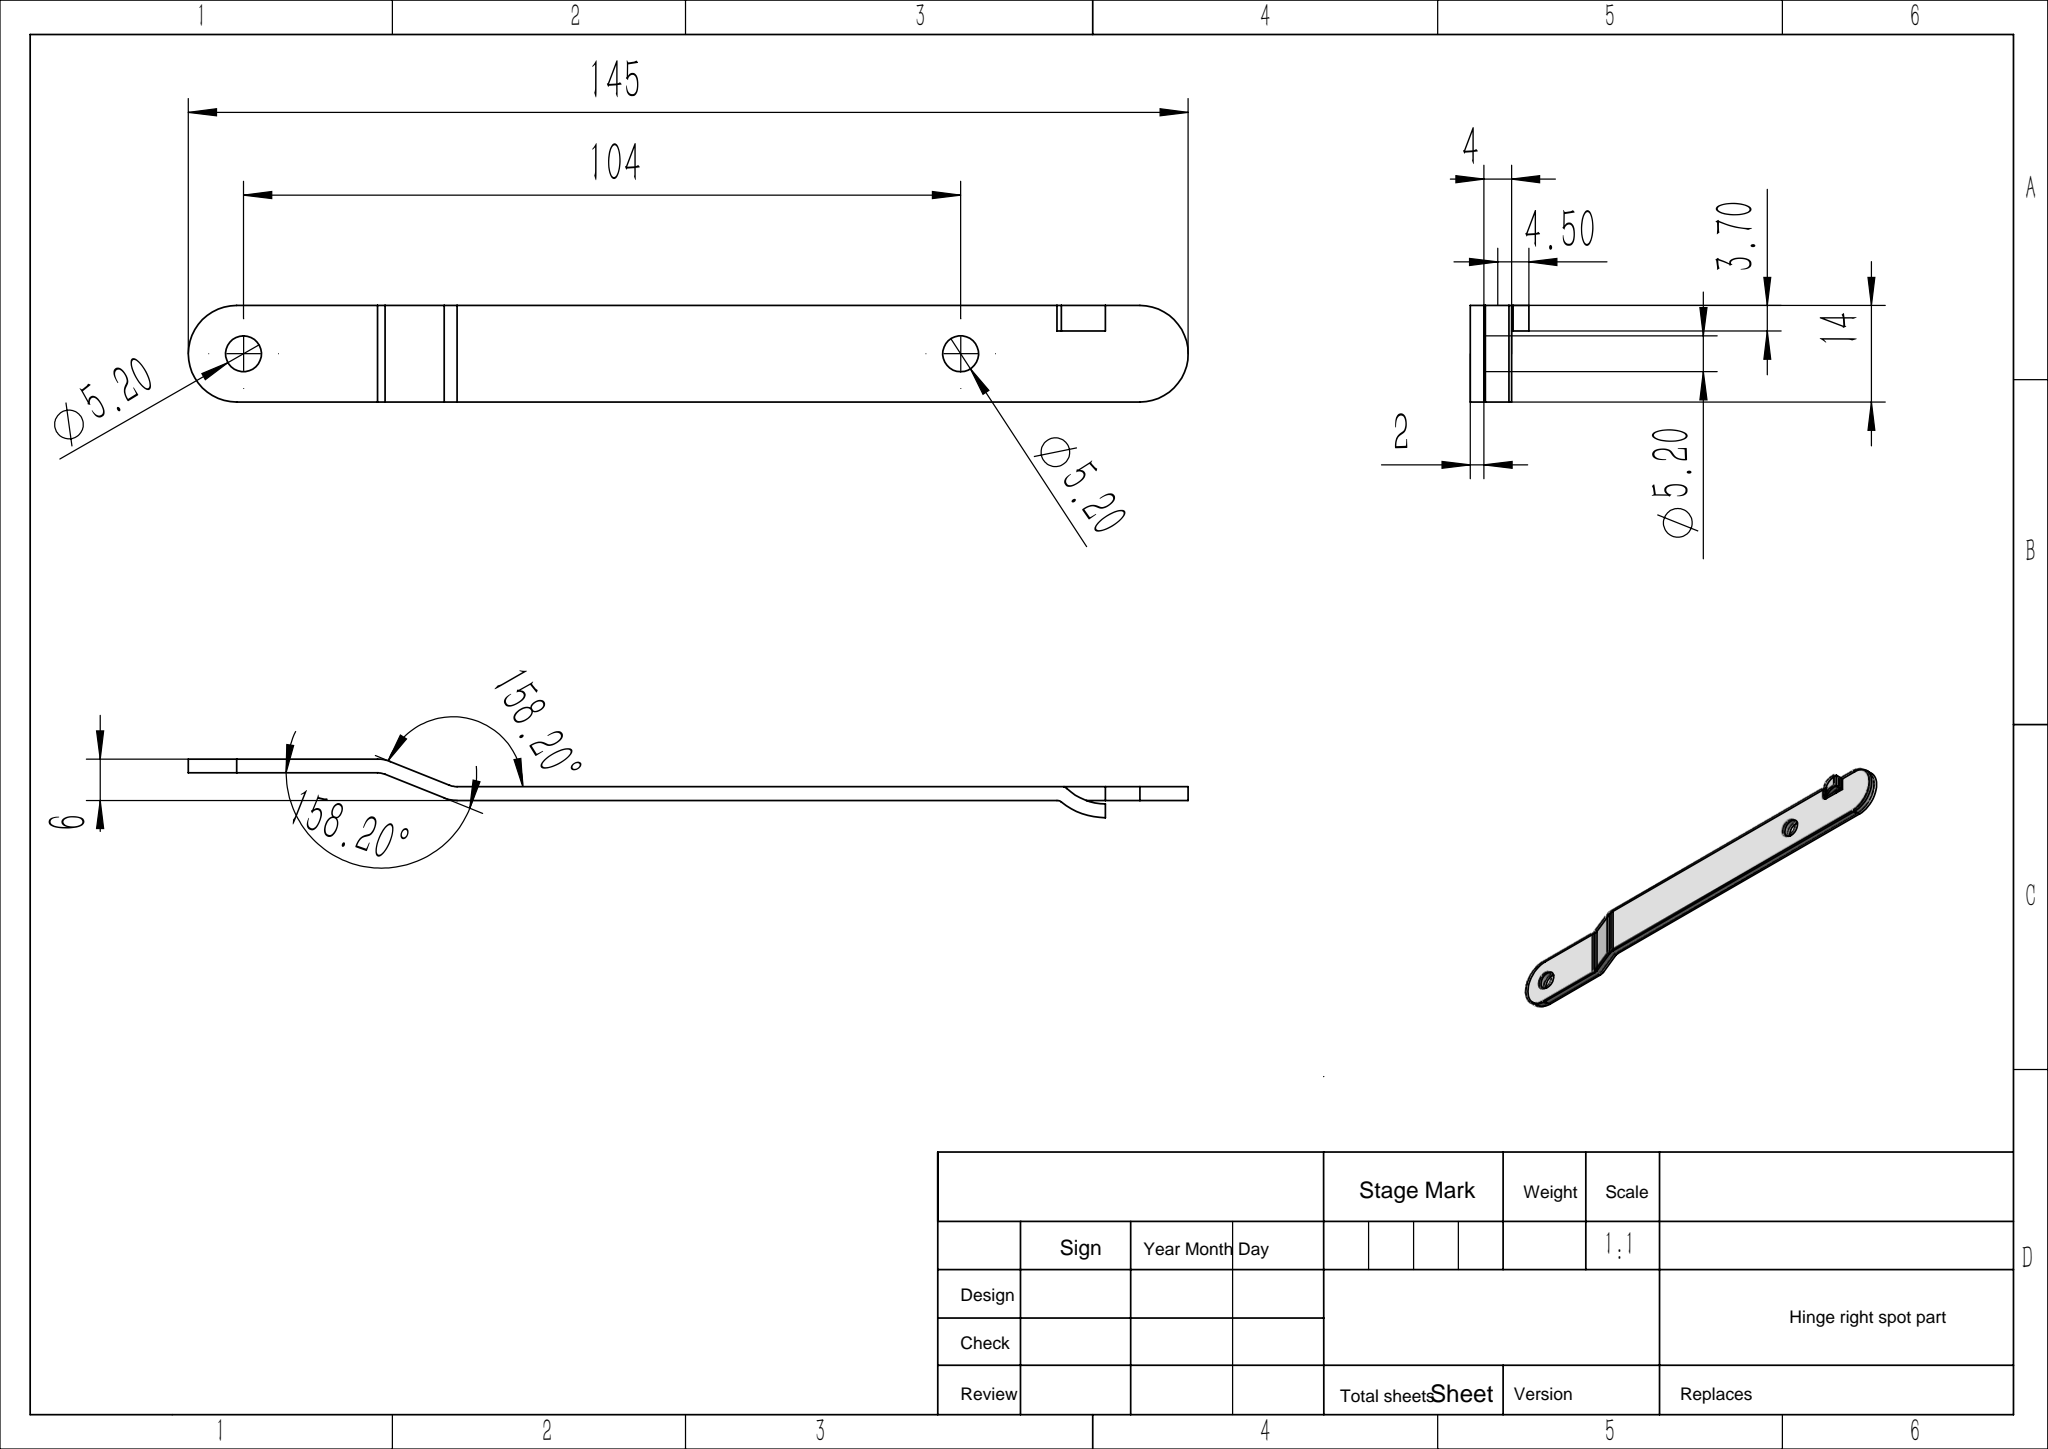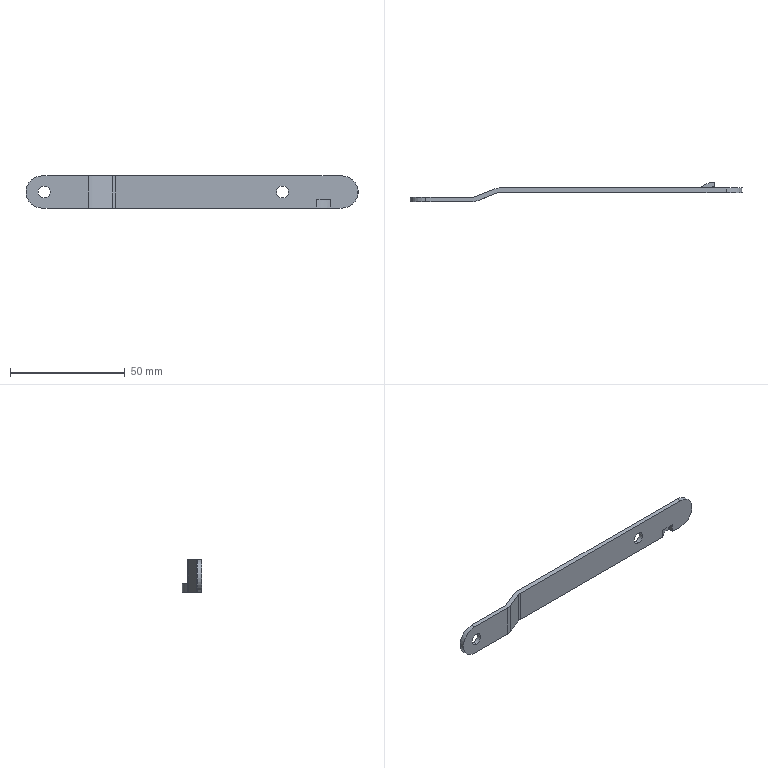Part | SolidWorks | features ICE 3, Extrusion 1 | 1 solid | 28 faces | box 145 x 8.5 x 14 mm | volume 3916 mm3 | cylinder 14 | plane 14 | commonest cylinder face diameters 5.2 x4 2 x2 6 x2 10 x2 14 x2 16.221 x1
STEP:
#1=CARTESIAN_POINT('',(112.,2.,-2.6));
#2=VERTEX_POINT('',#1);
#3=CARTESIAN_POINT('',(112.,2.,2.6));
#4=VERTEX_POINT('',#3);
#5=CARTESIAN_POINT('',(112.,2.,0.));
#6=DIRECTION('',(0.,1.,0.));
#7=DIRECTION('',(0.,0.,1.));
#8=AXIS2_PLACEMENT_3D('',#5,#6,#7);
#9=CIRCLE('',#8,2.6);
#10=EDGE_CURVE('',#2,#4,#9,.T.);
#11=ORIENTED_EDGE('',*,*,#10,.F.);
#12=CARTESIAN_POINT('',(112.,4.,-2.6));
#13=VERTEX_POINT('',#12);
#14=CARTESIAN_POINT('',(112.,-2.,-2.6));
#15=DIRECTION('',(0.,1.,0.));
#16=VECTOR('',#15,1000.);
#17=LINE('',#14,#16);
#18=EDGE_CURVE('',#2,#13,#17,.T.);
#19=ORIENTED_EDGE('',*,*,#18,.T.);
#20=CARTESIAN_POINT('',(112.,4.,2.6));
#21=VERTEX_POINT('',#20);
#22=CARTESIAN_POINT('',(112.,4.,0.));
#23=DIRECTION('',(0.,1.,0.));
#24=DIRECTION('',(0.,0.,1.));
#25=AXIS2_PLACEMENT_3D('',#22,#23,#24);
#26=CIRCLE('',#25,2.6);
#27=EDGE_CURVE('',#13,#21,#26,.T.);
#28=ORIENTED_EDGE('',*,*,#27,.T.);
#29=CARTESIAN_POINT('',(112.,-2.,2.6));
#30=DIRECTION('',(0.,1.,0.));
#31=VECTOR('',#30,1000.);
#32=LINE('',#29,#31);
#33=EDGE_CURVE('',#4,#21,#32,.T.);
#34=ORIENTED_EDGE('',*,*,#33,.F.);
#35=EDGE_LOOP('',(#11,#19,#28,#34));
#36=FACE_OUTER_BOUND('',#35,.T.);
#37=CARTESIAN_POINT('',(112.,-2.,0.));
#38=DIRECTION('',(0.,1.,0.));
#39=DIRECTION('',(0.,0.,1.));
#40=AXIS2_PLACEMENT_3D('',#37,#38,#39);
#41=CYLINDRICAL_SURFACE('',#40,2.6);
#42=ADVANCED_FACE('',(#36),#41,.F.);
#43=CARTESIAN_POINT('',(8.,-2.,-2.6));
#44=VERTEX_POINT('',#43);
#45=CARTESIAN_POINT('',(8.,-2.,2.6));
#46=VERTEX_POINT('',#45);
#47=CARTESIAN_POINT('',(8.,-2.,0.));
#48=DIRECTION('',(0.,1.,0.));
#49=DIRECTION('',(0.,0.,1.));
#50=AXIS2_PLACEMENT_3D('',#47,#48,#49);
#51=CIRCLE('',#50,2.6);
#52=EDGE_CURVE('',#44,#46,#51,.T.);
#53=ORIENTED_EDGE('',*,*,#52,.F.);
#54=CARTESIAN_POINT('',(8.,0.,-2.6));
#55=VERTEX_POINT('',#54);
#56=CARTESIAN_POINT('',(8.,-2.,-2.6));
#57=DIRECTION('',(0.,1.,0.));
#58=VECTOR('',#57,1000.);
#59=LINE('',#56,#58);
#60=EDGE_CURVE('',#44,#55,#59,.T.);
#61=ORIENTED_EDGE('',*,*,#60,.T.);
#62=CARTESIAN_POINT('',(8.,0.,2.6));
#63=VERTEX_POINT('',#62);
#64=CARTESIAN_POINT('',(8.,0.,0.));
#65=DIRECTION('',(0.,-1.,0.));
#66=DIRECTION('',(0.,0.,-1.));
#67=AXIS2_PLACEMENT_3D('',#64,#65,#66);
#68=CIRCLE('',#67,2.6);
#69=EDGE_CURVE('',#63,#55,#68,.T.);
#70=ORIENTED_EDGE('',*,*,#69,.F.);
#71=CARTESIAN_POINT('',(8.,-2.,2.6));
#72=DIRECTION('',(0.,1.,0.));
#73=VECTOR('',#72,1000.);
#74=LINE('',#71,#73);
#75=EDGE_CURVE('',#46,#63,#74,.T.);
#76=ORIENTED_EDGE('',*,*,#75,.F.);
#77=EDGE_LOOP('',(#53,#61,#70,#76));
#78=FACE_OUTER_BOUND('',#77,.T.);
#79=CARTESIAN_POINT('',(8.,-2.,0.));
#80=DIRECTION('',(0.,1.,0.));
#81=DIRECTION('',(0.,0.,1.));
#82=AXIS2_PLACEMENT_3D('',#79,#80,#81);
#83=CYLINDRICAL_SURFACE('',#82,2.6);
#84=ADVANCED_FACE('',(#78),#83,.F.);
#85=CARTESIAN_POINT('',(127.,2.037,-3.3));
#86=VERTEX_POINT('',#85);
#87=CARTESIAN_POINT('',(127.419,2.274,-3.3));
#88=VERTEX_POINT('',#87);
#89=CARTESIAN_POINT('',(126.731,3.,-3.3));
#90=DIRECTION('',(0.,0.,1.));
#91=DIRECTION('',(1.,0.,0.));
#92=AXIS2_PLACEMENT_3D('',#89,#90,#91);
#93=CIRCLE('',#92,1.);
#94=EDGE_CURVE('',#86,#88,#93,.T.);
#95=ORIENTED_EDGE('',*,*,#94,.T.);
#96=CARTESIAN_POINT('',(130.196,4.,-3.3));
#97=VERTEX_POINT('',#96);
#98=CARTESIAN_POINT('',(133.,-3.611,-3.3));
#99=DIRECTION('',(0.,0.,-1.));
#100=DIRECTION('',(-1.,0.,0.));
#101=AXIS2_PLACEMENT_3D('',#98,#99,#100);
#102=CIRCLE('',#101,8.111);
#103=EDGE_CURVE('',#88,#97,#102,.T.);
#104=ORIENTED_EDGE('',*,*,#103,.T.);
#105=CARTESIAN_POINT('',(133.,4.,-3.3));
#106=VERTEX_POINT('',#105);
#107=CARTESIAN_POINT('',(127.,4.,-3.3));
#108=DIRECTION('',(1.,0.,0.));
#109=VECTOR('',#108,1000.);
#110=LINE('',#107,#109);
#111=EDGE_CURVE('',#97,#106,#110,.T.);
#112=ORIENTED_EDGE('',*,*,#111,.T.);
#113=CARTESIAN_POINT('',(133.,2.,-3.3));
#114=VERTEX_POINT('',#113);
#115=CARTESIAN_POINT('',(133.,-2.,-3.3));
#116=DIRECTION('',(0.,1.,0.));
#117=VECTOR('',#116,1000.);
#118=LINE('',#115,#117);
#119=EDGE_CURVE('',#114,#106,#118,.T.);
#120=ORIENTED_EDGE('',*,*,#119,.F.);
#121=CARTESIAN_POINT('',(127.,2.,-3.3));
#122=VERTEX_POINT('',#121);
#123=CARTESIAN_POINT('',(38.963,2.,-3.3));
#124=DIRECTION('',(1.,0.,0.));
#125=VECTOR('',#124,1000.);
#126=LINE('',#123,#125);
#127=EDGE_CURVE('',#122,#114,#126,.T.);
#128=ORIENTED_EDGE('',*,*,#127,.F.);
#129=CARTESIAN_POINT('',(127.,-2.,-3.3));
#130=DIRECTION('',(0.,1.,0.));
#131=VECTOR('',#130,1000.);
#132=LINE('',#129,#131);
#133=EDGE_CURVE('',#122,#86,#132,.T.);
#134=ORIENTED_EDGE('',*,*,#133,.T.);
#135=EDGE_LOOP('',(#95,#104,#112,#120,#128,#134));
#136=FACE_OUTER_BOUND('',#135,.T.);
#137=CARTESIAN_POINT('',(127.,-2.,-3.3));
#138=DIRECTION('',(0.,0.,1.));
#139=DIRECTION('',(1.,0.,0.));
#140=AXIS2_PLACEMENT_3D('',#137,#138,#139);
#141=PLANE('',#140);
#142=ADVANCED_FACE('',(#136),#141,.F.);
#143=CARTESIAN_POINT('',(127.,2.037,-7.));
#144=VERTEX_POINT('',#143);
#145=CARTESIAN_POINT('',(127.,2.037,-3.3));
#146=DIRECTION('',(0.,0.,-1.));
#147=VECTOR('',#146,1000.);
#148=LINE('',#145,#147);
#149=EDGE_CURVE('',#86,#144,#148,.T.);
#150=ORIENTED_EDGE('',*,*,#149,.F.);
#151=ORIENTED_EDGE('',*,*,#133,.F.);
#152=CARTESIAN_POINT('',(127.,2.,-7.));
#153=VERTEX_POINT('',#152);
#154=CARTESIAN_POINT('',(127.,2.,7.));
#155=DIRECTION('',(0.,0.,1.));
#156=VECTOR('',#155,1000.);
#157=LINE('',#154,#156);
#158=EDGE_CURVE('',#153,#122,#157,.T.);
#159=ORIENTED_EDGE('',*,*,#158,.F.);
#160=CARTESIAN_POINT('',(127.,3.,-7.));
#161=DIRECTION('',(0.,1.,0.));
#162=VECTOR('',#161,1000.);
#163=LINE('',#160,#162);
#164=EDGE_CURVE('',#153,#144,#163,.T.);
#165=ORIENTED_EDGE('',*,*,#164,.T.);
#166=EDGE_LOOP('',(#150,#151,#159,#165));
#167=FACE_OUTER_BOUND('',#166,.T.);
#168=CARTESIAN_POINT('',(127.,-2.,-7.));
#169=DIRECTION('',(-1.,0.,0.));
#170=DIRECTION('',(0.,0.,1.));
#171=AXIS2_PLACEMENT_3D('',#168,#169,#170);
#172=PLANE('',#171);
#173=ADVANCED_FACE('',(#167),#172,.F.);
#174=CARTESIAN_POINT('',(125.978,4.,-7.));
#175=VERTEX_POINT('',#174);
#176=CARTESIAN_POINT('',(38.963,4.,-7.));
#177=VERTEX_POINT('',#176);
#178=CARTESIAN_POINT('',(38.963,4.,-7.));
#179=DIRECTION('',(-1.,0.,0.));
#180=VECTOR('',#179,1000.);
#181=LINE('',#178,#180);
#182=EDGE_CURVE('',#175,#177,#181,.T.);
#183=ORIENTED_EDGE('',*,*,#182,.F.);
#184=CARTESIAN_POINT('',(126.61,4.225,-7.));
#185=VERTEX_POINT('',#184);
#186=CARTESIAN_POINT('',(125.978,5.,-7.));
#187=DIRECTION('',(0.,0.,-1.));
#188=DIRECTION('',(1.,0.,0.));
#189=AXIS2_PLACEMENT_3D('',#186,#187,#188);
#190=CIRCLE('',#189,1.);
#191=EDGE_CURVE('',#185,#175,#190,.T.);
#192=ORIENTED_EDGE('',*,*,#191,.F.);
#193=CARTESIAN_POINT('',(133.,6.5,-7.));
#194=VERTEX_POINT('',#193);
#195=CARTESIAN_POINT('',(133.,-3.611,-7.));
#196=DIRECTION('',(0.,0.,1.));
#197=DIRECTION('',(-1.,0.,0.));
#198=AXIS2_PLACEMENT_3D('',#195,#196,#197);
#199=CIRCLE('',#198,10.111);
#200=EDGE_CURVE('',#194,#185,#199,.T.);
#201=ORIENTED_EDGE('',*,*,#200,.F.);
#202=CARTESIAN_POINT('',(133.,4.5,-7.));
#203=VERTEX_POINT('',#202);
#204=CARTESIAN_POINT('',(133.,4.5,-7.));
#205=DIRECTION('',(0.,1.,0.));
#206=VECTOR('',#205,1000.);
#207=LINE('',#204,#206);
#208=EDGE_CURVE('',#203,#194,#207,.T.);
#209=ORIENTED_EDGE('',*,*,#208,.F.);
#210=CARTESIAN_POINT('',(127.419,2.274,-7.));
#211=VERTEX_POINT('',#210);
#212=CARTESIAN_POINT('',(133.,-3.611,-7.));
#213=DIRECTION('',(0.,0.,-1.));
#214=DIRECTION('',(-1.,0.,0.));
#215=AXIS2_PLACEMENT_3D('',#212,#213,#214);
#216=CIRCLE('',#215,8.111);
#217=EDGE_CURVE('',#211,#203,#216,.T.);
#218=ORIENTED_EDGE('',*,*,#217,.F.);
#219=CARTESIAN_POINT('',(126.731,3.,-7.));
#220=DIRECTION('',(0.,0.,1.));
#221=DIRECTION('',(1.,0.,0.));
#222=AXIS2_PLACEMENT_3D('',#219,#220,#221);
#223=CIRCLE('',#222,1.);
#224=EDGE_CURVE('',#144,#211,#223,.T.);
#225=ORIENTED_EDGE('',*,*,#224,.F.);
#226=ORIENTED_EDGE('',*,*,#164,.F.);
#227=CARTESIAN_POINT('',(38.963,2.,-7.));
#228=VERTEX_POINT('',#227);
#229=CARTESIAN_POINT('',(38.963,2.,-7.));
#230=DIRECTION('',(1.,0.,0.));
#231=VECTOR('',#230,1000.);
#232=LINE('',#229,#231);
#233=EDGE_CURVE('',#228,#153,#232,.T.);
#234=ORIENTED_EDGE('',*,*,#233,.F.);
#235=CARTESIAN_POINT('',(37.849,1.785,-7.));
#236=VERTEX_POINT('',#235);
#237=CARTESIAN_POINT('',(38.963,-1.,-7.));
#238=DIRECTION('',(0.,0.,-1.));
#239=DIRECTION('',(1.,0.,0.));
#240=AXIS2_PLACEMENT_3D('',#237,#238,#239);
#241=CIRCLE('',#240,3.);
#242=EDGE_CURVE('',#236,#228,#241,.T.);
#243=ORIENTED_EDGE('',*,*,#242,.F.);
#244=CARTESIAN_POINT('',(29.279,-1.642,-7.));
#245=VERTEX_POINT('',#244);
#246=CARTESIAN_POINT('',(29.279,-1.642,-7.));
#247=DIRECTION('',(0.9285,0.3714,0.));
#248=VECTOR('',#247,1000.);
#249=LINE('',#246,#248);
#250=EDGE_CURVE('',#245,#236,#249,.T.);
#251=ORIENTED_EDGE('',*,*,#250,.F.);
#252=CARTESIAN_POINT('',(27.422,-2.,-7.));
#253=VERTEX_POINT('',#252);
#254=CARTESIAN_POINT('',(27.422,3.,-7.));
#255=DIRECTION('',(0.,0.,1.));
#256=DIRECTION('',(-1.,0.,0.));
#257=AXIS2_PLACEMENT_3D('',#254,#255,#256);
#258=CIRCLE('',#257,5.);
#259=EDGE_CURVE('',#253,#245,#258,.T.);
#260=ORIENTED_EDGE('',*,*,#259,.F.);
#261=CARTESIAN_POINT('',(7.,-2.,-7.));
#262=VERTEX_POINT('',#261);
#263=CARTESIAN_POINT('',(0.,-2.,-7.));
#264=DIRECTION('',(1.,0.,0.));
#265=VECTOR('',#264,1000.);
#266=LINE('',#263,#265);
#267=EDGE_CURVE('',#262,#253,#266,.T.);
#268=ORIENTED_EDGE('',*,*,#267,.F.);
#269=CARTESIAN_POINT('',(7.,0.,-7.));
#270=VERTEX_POINT('',#269);
#271=CARTESIAN_POINT('',(7.,-2.,-7.));
#272=DIRECTION('',(0.,1.,0.));
#273=VECTOR('',#272,1000.);
#274=LINE('',#271,#273);
#275=EDGE_CURVE('',#262,#270,#274,.T.);
#276=ORIENTED_EDGE('',*,*,#275,.T.);
#277=CARTESIAN_POINT('',(27.422,0.,-7.));
#278=VERTEX_POINT('',#277);
#279=CARTESIAN_POINT('',(0.,0.,-7.));
#280=DIRECTION('',(-1.,0.,0.));
#281=VECTOR('',#280,1000.);
#282=LINE('',#279,#281);
#283=EDGE_CURVE('',#278,#270,#282,.T.);
#284=ORIENTED_EDGE('',*,*,#283,.F.);
#285=CARTESIAN_POINT('',(28.536,0.2146,-7.));
#286=VERTEX_POINT('',#285);
#287=CARTESIAN_POINT('',(27.422,3.,-7.));
#288=DIRECTION('',(0.,0.,-1.));
#289=DIRECTION('',(-1.,0.,0.));
#290=AXIS2_PLACEMENT_3D('',#287,#288,#289);
#291=CIRCLE('',#290,3.);
#292=EDGE_CURVE('',#286,#278,#291,.T.);
#293=ORIENTED_EDGE('',*,*,#292,.F.);
#294=CARTESIAN_POINT('',(37.106,3.642,-7.));
#295=VERTEX_POINT('',#294);
#296=CARTESIAN_POINT('',(28.536,0.2146,-7.));
#297=DIRECTION('',(-0.9285,-0.3714,0.));
#298=VECTOR('',#297,1000.);
#299=LINE('',#296,#298);
#300=EDGE_CURVE('',#295,#286,#299,.T.);
#301=ORIENTED_EDGE('',*,*,#300,.F.);
#302=CARTESIAN_POINT('',(38.963,-1.,-7.));
#303=DIRECTION('',(0.,0.,1.));
#304=DIRECTION('',(1.,0.,0.));
#305=AXIS2_PLACEMENT_3D('',#302,#303,#304);
#306=CIRCLE('',#305,5.);
#307=EDGE_CURVE('',#177,#295,#306,.T.);
#308=ORIENTED_EDGE('',*,*,#307,.F.);
#309=EDGE_LOOP('',(#183,#192,#201,#209,#218,#225,#226,#234,#243,#251,#260,#268,#276,#284,#293,#301,#308));
#310=FACE_OUTER_BOUND('',#309,.T.);
#311=CARTESIAN_POINT('',(27.422,3.,-7.));
#312=DIRECTION('',(0.,0.,-1.));
#313=DIRECTION('',(-1.,0.,0.));
#314=AXIS2_PLACEMENT_3D('',#311,#312,#313);
#315=PLANE('',#314);
#316=ADVANCED_FACE('',(#310),#315,.T.);
#317=CARTESIAN_POINT('',(8.,-2.,0.));
#318=DIRECTION('',(0.,1.,0.));
#319=DIRECTION('',(0.,0.,1.));
#320=AXIS2_PLACEMENT_3D('',#317,#318,#319);
#321=CIRCLE('',#320,2.6);
#322=EDGE_CURVE('',#46,#44,#321,.T.);
#323=ORIENTED_EDGE('',*,*,#322,.T.);
#324=ORIENTED_EDGE('',*,*,#52,.T.);
#325=EDGE_LOOP('',(#323,#324));
#326=FACE_BOUND('',#325,.T.);
#327=CARTESIAN_POINT('',(7.,-2.,7.));
#328=VERTEX_POINT('',#327);
#329=CARTESIAN_POINT('',(27.422,-2.,7.));
#330=VERTEX_POINT('',#329);
#331=CARTESIAN_POINT('',(0.,-2.,7.));
#332=DIRECTION('',(1.,0.,0.));
#333=VECTOR('',#332,1000.);
#334=LINE('',#331,#333);
#335=EDGE_CURVE('',#328,#330,#334,.T.);
#336=ORIENTED_EDGE('',*,*,#335,.F.);
#337=CARTESIAN_POINT('',(7.,-2.,0.));
#338=DIRECTION('',(0.,-1.,0.));
#339=DIRECTION('',(0.,0.,1.));
#340=AXIS2_PLACEMENT_3D('',#337,#338,#339);
#341=CIRCLE('',#340,7.);
#342=EDGE_CURVE('',#328,#262,#341,.T.);
#343=ORIENTED_EDGE('',*,*,#342,.T.);
#344=ORIENTED_EDGE('',*,*,#267,.T.);
#345=CARTESIAN_POINT('',(27.422,-2.,7.));
#346=DIRECTION('',(0.,0.,-1.));
#347=VECTOR('',#346,1000.);
#348=LINE('',#345,#347);
#349=EDGE_CURVE('',#330,#253,#348,.T.);
#350=ORIENTED_EDGE('',*,*,#349,.F.);
#351=EDGE_LOOP('',(#336,#343,#344,#350));
#352=FACE_OUTER_BOUND('',#351,.T.);
#353=CARTESIAN_POINT('',(0.,-2.,7.));
#354=DIRECTION('',(0.,1.,0.));
#355=DIRECTION('',(0.,0.,1.));
#356=AXIS2_PLACEMENT_3D('',#353,#354,#355);
#357=PLANE('',#356);
#358=ADVANCED_FACE('',(#326,#352),#357,.F.);
#359=ORIENTED_EDGE('',*,*,#259,.T.);
#360=CARTESIAN_POINT('',(29.279,-1.642,7.));
#361=VERTEX_POINT('',#360);
#362=CARTESIAN_POINT('',(29.279,-1.642,7.));
#363=DIRECTION('',(0.,0.,-1.));
#364=VECTOR('',#363,1000.);
#365=LINE('',#362,#364);
#366=EDGE_CURVE('',#361,#245,#365,.T.);
#367=ORIENTED_EDGE('',*,*,#366,.F.);
#368=CARTESIAN_POINT('',(27.422,3.,7.));
#369=DIRECTION('',(0.,0.,1.));
#370=DIRECTION('',(-1.,0.,0.));
#371=AXIS2_PLACEMENT_3D('',#368,#369,#370);
#372=CIRCLE('',#371,5.);
#373=EDGE_CURVE('',#330,#361,#372,.T.);
#374=ORIENTED_EDGE('',*,*,#373,.F.);
#375=ORIENTED_EDGE('',*,*,#349,.T.);
#376=EDGE_LOOP('',(#359,#367,#374,#375));
#377=FACE_OUTER_BOUND('',#376,.T.);
#378=CARTESIAN_POINT('',(27.422,3.,7.));
#379=DIRECTION('',(0.,0.,-1.));
#380=DIRECTION('',(-1.,0.,0.));
#381=AXIS2_PLACEMENT_3D('',#378,#379,#380);
#382=CYLINDRICAL_SURFACE('',#381,5.);
#383=ADVANCED_FACE('',(#377),#382,.T.);
#384=ORIENTED_EDGE('',*,*,#250,.T.);
#385=CARTESIAN_POINT('',(37.849,1.785,7.));
#386=VERTEX_POINT('',#385);
#387=CARTESIAN_POINT('',(37.849,1.785,7.));
#388=DIRECTION('',(0.,0.,-1.));
#389=VECTOR('',#388,1000.);
#390=LINE('',#387,#389);
#391=EDGE_CURVE('',#386,#236,#390,.T.);
#392=ORIENTED_EDGE('',*,*,#391,.F.);
#393=CARTESIAN_POINT('',(29.279,-1.642,7.));
#394=DIRECTION('',(0.9285,0.3714,0.));
#395=VECTOR('',#394,1000.);
#396=LINE('',#393,#395);
#397=EDGE_CURVE('',#361,#386,#396,.T.);
#398=ORIENTED_EDGE('',*,*,#397,.F.);
#399=ORIENTED_EDGE('',*,*,#366,.T.);
#400=EDGE_LOOP('',(#384,#392,#398,#399));
#401=FACE_OUTER_BOUND('',#400,.T.);
#402=CARTESIAN_POINT('',(29.279,-1.642,7.));
#403=DIRECTION('',(-0.3714,0.9285,0.));
#404=DIRECTION('',(-0.9285,-0.3714,0.));
#405=AXIS2_PLACEMENT_3D('',#402,#403,#404);
#406=PLANE('',#405);
#407=ADVANCED_FACE('',(#401),#406,.F.);
#408=ORIENTED_EDGE('',*,*,#242,.T.);
#409=CARTESIAN_POINT('',(38.963,2.,7.));
#410=VERTEX_POINT('',#409);
#411=CARTESIAN_POINT('',(38.963,2.,7.));
#412=DIRECTION('',(0.,0.,-1.));
#413=VECTOR('',#412,1000.);
#414=LINE('',#411,#413);
#415=EDGE_CURVE('',#410,#228,#414,.T.);
#416=ORIENTED_EDGE('',*,*,#415,.F.);
#417=CARTESIAN_POINT('',(38.963,-1.,7.));
#418=DIRECTION('',(0.,0.,-1.));
#419=DIRECTION('',(1.,0.,0.));
#420=AXIS2_PLACEMENT_3D('',#417,#418,#419);
#421=CIRCLE('',#420,3.);
#422=EDGE_CURVE('',#386,#410,#421,.T.);
#423=ORIENTED_EDGE('',*,*,#422,.F.);
#424=ORIENTED_EDGE('',*,*,#391,.T.);
#425=EDGE_LOOP('',(#408,#416,#423,#424));
#426=FACE_OUTER_BOUND('',#425,.T.);
#427=CARTESIAN_POINT('',(38.963,-1.,7.));
#428=DIRECTION('',(0.,0.,-1.));
#429=DIRECTION('',(-1.,0.,0.));
#430=AXIS2_PLACEMENT_3D('',#427,#428,#429);
#431=CYLINDRICAL_SURFACE('',#430,3.);
#432=ADVANCED_FACE('',(#426),#431,.F.);
#433=ORIENTED_EDGE('',*,*,#233,.T.);
#434=ORIENTED_EDGE('',*,*,#158,.T.);
#435=ORIENTED_EDGE('',*,*,#127,.T.);
#436=CARTESIAN_POINT('',(133.,2.,-7.));
#437=VERTEX_POINT('',#436);
#438=CARTESIAN_POINT('',(133.,2.,7.));
#439=DIRECTION('',(0.,0.,-1.));
#440=VECTOR('',#439,1000.);
#441=LINE('',#438,#440);
#442=EDGE_CURVE('',#114,#437,#441,.T.);
#443=ORIENTED_EDGE('',*,*,#442,.T.);
#444=CARTESIAN_POINT('',(138.,2.,-7.));
#445=VERTEX_POINT('',#444);
#446=CARTESIAN_POINT('',(38.963,2.,-7.));
#447=DIRECTION('',(1.,0.,0.));
#448=VECTOR('',#447,1000.);
#449=LINE('',#446,#448);
#450=EDGE_CURVE('',#437,#445,#449,.T.);
#451=ORIENTED_EDGE('',*,*,#450,.T.);
#452=CARTESIAN_POINT('',(138.,2.,7.));
#453=VERTEX_POINT('',#452);
#454=CARTESIAN_POINT('',(138.,2.,0.));
#455=DIRECTION('',(0.,-1.,0.));
#456=DIRECTION('',(0.,0.,1.));
#457=AXIS2_PLACEMENT_3D('',#454,#455,#456);
#458=CIRCLE('',#457,7.);
#459=EDGE_CURVE('',#445,#453,#458,.T.);
#460=ORIENTED_EDGE('',*,*,#459,.T.);
#461=CARTESIAN_POINT('',(38.963,2.,7.));
#462=DIRECTION('',(1.,0.,0.));
#463=VECTOR('',#462,1000.);
#464=LINE('',#461,#463);
#465=EDGE_CURVE('',#410,#453,#464,.T.);
#466=ORIENTED_EDGE('',*,*,#465,.F.);
#467=ORIENTED_EDGE('',*,*,#415,.T.);
#468=EDGE_LOOP('',(#433,#434,#435,#443,#451,#460,#466,#467));
#469=FACE_OUTER_BOUND('',#468,.T.);
#470=CARTESIAN_POINT('',(112.,2.,0.));
#471=DIRECTION('',(0.,1.,0.));
#472=DIRECTION('',(0.,0.,1.));
#473=AXIS2_PLACEMENT_3D('',#470,#471,#472);
#474=CIRCLE('',#473,2.6);
#475=EDGE_CURVE('',#4,#2,#474,.T.);
#476=ORIENTED_EDGE('',*,*,#475,.T.);
#477=ORIENTED_EDGE('',*,*,#10,.T.);
#478=EDGE_LOOP('',(#476,#477));
#479=FACE_BOUND('',#478,.T.);
#480=CARTESIAN_POINT('',(38.963,2.,7.));
#481=DIRECTION('',(0.,1.,0.));
#482=DIRECTION('',(0.,0.,1.));
#483=AXIS2_PLACEMENT_3D('',#480,#481,#482);
#484=PLANE('',#483);
#485=ADVANCED_FACE('',(#469,#479),#484,.F.);
#486=ORIENTED_EDGE('',*,*,#182,.T.);
#487=CARTESIAN_POINT('',(38.963,4.,7.));
#488=VERTEX_POINT('',#487);
#489=CARTESIAN_POINT('',(38.963,4.,7.));
#490=DIRECTION('',(0.,0.,-1.));
#491=VECTOR('',#490,1000.);
#492=LINE('',#489,#491);
#493=EDGE_CURVE('',#488,#177,#492,.T.);
#494=ORIENTED_EDGE('',*,*,#493,.F.);
#495=CARTESIAN_POINT('',(138.,4.,7.));
#496=VERTEX_POINT('',#495);
#497=CARTESIAN_POINT('',(38.963,4.,7.));
#498=DIRECTION('',(-1.,0.,0.));
#499=VECTOR('',#498,1000.);
#500=LINE('',#497,#499);
#501=EDGE_CURVE('',#496,#488,#500,.T.);
#502=ORIENTED_EDGE('',*,*,#501,.F.);
#503=CARTESIAN_POINT('',(138.,4.,-7.));
#504=VERTEX_POINT('',#503);
#505=CARTESIAN_POINT('',(138.,4.,0.));
#506=DIRECTION('',(0.,-1.,0.));
#507=DIRECTION('',(0.,0.,1.));
#508=AXIS2_PLACEMENT_3D('',#505,#506,#507);
#509=CIRCLE('',#508,7.);
#510=EDGE_CURVE('',#504,#496,#509,.T.);
#511=ORIENTED_EDGE('',*,*,#510,.F.);
#512=CARTESIAN_POINT('',(133.,4.,-7.));
#513=VERTEX_POINT('',#512);
#514=CARTESIAN_POINT('',(38.963,4.,-7.));
#515=DIRECTION('',(-1.,0.,0.));
#516=VECTOR('',#515,1000.);
#517=LINE('',#514,#516);
#518=EDGE_CURVE('',#504,#513,#517,.T.);
#519=ORIENTED_EDGE('',*,*,#518,.T.);
#520=CARTESIAN_POINT('',(133.,4.,-7.));
#521=DIRECTION('',(0.,0.,-1.));
#522=VECTOR('',#521,1000.);
#523=LINE('',#520,#522);
#524=EDGE_CURVE('',#106,#513,#523,.T.);
#525=ORIENTED_EDGE('',*,*,#524,.F.);
#526=ORIENTED_EDGE('',*,*,#111,.F.);
#527=CARTESIAN_POINT('',(125.978,4.,-3.3));
#528=VERTEX_POINT('',#527);
#529=CARTESIAN_POINT('',(127.,4.,-3.3));
#530=DIRECTION('',(1.,0.,0.));
#531=VECTOR('',#530,1000.);
#532=LINE('',#529,#531);
#533=EDGE_CURVE('',#528,#97,#532,.T.);
#534=ORIENTED_EDGE('',*,*,#533,.F.);
#535=CARTESIAN_POINT('',(125.978,4.,-3.3));
#536=DIRECTION('',(0.,0.,-1.));
#537=VECTOR('',#536,1000.);
#538=LINE('',#535,#537);
#539=EDGE_CURVE('',#528,#175,#538,.T.);
#540=ORIENTED_EDGE('',*,*,#539,.T.);
#541=EDGE_LOOP('',(#486,#494,#502,#511,#519,#525,#526,#534,#540));
#542=FACE_OUTER_BOUND('',#541,.T.);
#543=CARTESIAN_POINT('',(112.,4.,0.));
#544=DIRECTION('',(0.,1.,0.));
#545=DIRECTION('',(0.,0.,1.));
#546=AXIS2_PLACEMENT_3D('',#543,#544,#545);
#547=CIRCLE('',#546,2.6);
#548=EDGE_CURVE('',#21,#13,#547,.T.);
#549=ORIENTED_EDGE('',*,*,#548,.F.);
#550=ORIENTED_EDGE('',*,*,#27,.F.);
#551=EDGE_LOOP('',(#549,#550));
#552=FACE_BOUND('',#551,.T.);
#553=CARTESIAN_POINT('',(38.963,4.,7.));
#554=DIRECTION('',(0.,-1.,0.));
#555=DIRECTION('',(0.,0.,-1.));
#556=AXIS2_PLACEMENT_3D('',#553,#554,#555);
#557=PLANE('',#556);
#558=ADVANCED_FACE('',(#542,#552),#557,.F.);
#559=ORIENTED_EDGE('',*,*,#307,.T.);
#560=CARTESIAN_POINT('',(37.106,3.642,7.));
#561=VERTEX_POINT('',#560);
#562=CARTESIAN_POINT('',(37.106,3.642,7.));
#563=DIRECTION('',(0.,0.,-1.));
#564=VECTOR('',#563,1000.);
#565=LINE('',#562,#564);
#566=EDGE_CURVE('',#561,#295,#565,.T.);
#567=ORIENTED_EDGE('',*,*,#566,.F.);
#568=CARTESIAN_POINT('',(38.963,-1.,7.));
#569=DIRECTION('',(0.,0.,1.));
#570=DIRECTION('',(1.,0.,0.));
#571=AXIS2_PLACEMENT_3D('',#568,#569,#570);
#572=CIRCLE('',#571,5.);
#573=EDGE_CURVE('',#488,#561,#572,.T.);
#574=ORIENTED_EDGE('',*,*,#573,.F.);
#575=ORIENTED_EDGE('',*,*,#493,.T.);
#576=EDGE_LOOP('',(#559,#567,#574,#575));
#577=FACE_OUTER_BOUND('',#576,.T.);
#578=CARTESIAN_POINT('',(38.963,-1.,7.));
#579=DIRECTION('',(0.,0.,-1.));
#580=DIRECTION('',(-1.,0.,0.));
#581=AXIS2_PLACEMENT_3D('',#578,#579,#580);
#582=CYLINDRICAL_SURFACE('',#581,5.);
#583=ADVANCED_FACE('',(#577),#582,.T.);
#584=ORIENTED_EDGE('',*,*,#300,.T.);
#585=CARTESIAN_POINT('',(28.536,0.2146,7.));
#586=VERTEX_POINT('',#585);
#587=CARTESIAN_POINT('',(28.536,0.2146,7.));
#588=DIRECTION('',(0.,0.,-1.));
#589=VECTOR('',#588,1000.);
#590=LINE('',#587,#589);
#591=EDGE_CURVE('',#586,#286,#590,.T.);
#592=ORIENTED_EDGE('',*,*,#591,.F.);
#593=CARTESIAN_POINT('',(28.536,0.2146,7.));
#594=DIRECTION('',(-0.9285,-0.3714,0.));
#595=VECTOR('',#594,1000.);
#596=LINE('',#593,#595);
#597=EDGE_CURVE('',#561,#586,#596,.T.);
#598=ORIENTED_EDGE('',*,*,#597,.F.);
#599=ORIENTED_EDGE('',*,*,#566,.T.);
#600=EDGE_LOOP('',(#584,#592,#598,#599));
#601=FACE_OUTER_BOUND('',#600,.T.);
#602=CARTESIAN_POINT('',(28.536,0.2146,7.));
#603=DIRECTION('',(0.3714,-0.9285,0.));
#604=DIRECTION('',(0.9285,0.3714,0.));
#605=AXIS2_PLACEMENT_3D('',#602,#603,#604);
#606=PLANE('',#605);
#607=ADVANCED_FACE('',(#601),#606,.F.);
#608=ORIENTED_EDGE('',*,*,#292,.T.);
#609=CARTESIAN_POINT('',(27.422,0.,7.));
#610=VERTEX_POINT('',#609);
#611=CARTESIAN_POINT('',(27.422,0.,7.));
#612=DIRECTION('',(0.,0.,-1.));
#613=VECTOR('',#612,1000.);
#614=LINE('',#611,#613);
#615=EDGE_CURVE('',#610,#278,#614,.T.);
#616=ORIENTED_EDGE('',*,*,#615,.F.);
#617=CARTESIAN_POINT('',(27.422,3.,7.));
#618=DIRECTION('',(0.,0.,-1.));
#619=DIRECTION('',(-1.,0.,0.));
#620=AXIS2_PLACEMENT_3D('',#617,#618,#619);
#621=CIRCLE('',#620,3.);
#622=EDGE_CURVE('',#586,#610,#621,.T.);
#623=ORIENTED_EDGE('',*,*,#622,.F.);
#624=ORIENTED_EDGE('',*,*,#591,.T.);
#625=EDGE_LOOP('',(#608,#616,#623,#624));
#626=FACE_OUTER_BOUND('',#625,.T.);
#627=CARTESIAN_POINT('',(27.422,3.,7.));
#628=DIRECTION('',(0.,0.,-1.));
#629=DIRECTION('',(-1.,0.,0.));
#630=AXIS2_PLACEMENT_3D('',#627,#628,#629);
#631=CYLINDRICAL_SURFACE('',#630,3.);
#632=ADVANCED_FACE('',(#626),#631,.F.);
#633=ORIENTED_EDGE('',*,*,#69,.T.);
#634=CARTESIAN_POINT('',(8.,0.,0.));
#635=DIRECTION('',(0.,-1.,0.));
#636=DIRECTION('',(0.,0.,-1.));
#637=AXIS2_PLACEMENT_3D('',#634,#635,#636);
#638=CIRCLE('',#637,2.6);
#639=EDGE_CURVE('',#55,#63,#638,.T.);
#640=ORIENTED_EDGE('',*,*,#639,.T.);
#641=EDGE_LOOP('',(#633,#640));
#642=FACE_BOUND('',#641,.T.);
#643=ORIENTED_EDGE('',*,*,#283,.T.);
#644=CARTESIAN_POINT('',(7.,0.,7.));
#645=VERTEX_POINT('',#644);
#646=CARTESIAN_POINT('',(7.,0.,0.));
#647=DIRECTION('',(0.,1.,0.));
#648=DIRECTION('',(0.,0.,-1.));
#649=AXIS2_PLACEMENT_3D('',#646,#647,#648);
#650=CIRCLE('',#649,7.);
#651=EDGE_CURVE('',#270,#645,#650,.T.);
#652=ORIENTED_EDGE('',*,*,#651,.T.);
#653=CARTESIAN_POINT('',(0.,0.,7.));
#654=DIRECTION('',(-1.,0.,0.));
#655=VECTOR('',#654,1000.);
#656=LINE('',#653,#655);
#657=EDGE_CURVE('',#610,#645,#656,.T.);
#658=ORIENTED_EDGE('',*,*,#657,.F.);
#659=ORIENTED_EDGE('',*,*,#615,.T.);
#660=EDGE_LOOP('',(#643,#652,#658,#659));
#661=FACE_OUTER_BOUND('',#660,.T.);
#662=CARTESIAN_POINT('',(0.,0.,7.));
#663=DIRECTION('',(0.,-1.,0.));
#664=DIRECTION('',(0.,0.,-1.));
#665=AXIS2_PLACEMENT_3D('',#662,#663,#664);
#666=PLANE('',#665);
#667=ADVANCED_FACE('',(#642,#661),#666,.F.);
#668=ORIENTED_EDGE('',*,*,#465,.T.);
#669=CARTESIAN_POINT('',(138.,-2.,7.));
#670=DIRECTION('',(0.,1.,0.));
#671=VECTOR('',#670,1000.);
#672=LINE('',#669,#671);
#673=EDGE_CURVE('',#453,#496,#672,.T.);
#674=ORIENTED_EDGE('',*,*,#673,.T.);
#675=ORIENTED_EDGE('',*,*,#501,.T.);
#676=ORIENTED_EDGE('',*,*,#573,.T.);
#677=ORIENTED_EDGE('',*,*,#597,.T.);
#678=ORIENTED_EDGE('',*,*,#622,.T.);
#679=ORIENTED_EDGE('',*,*,#657,.T.);
#680=CARTESIAN_POINT('',(7.,-2.,7.));
#681=DIRECTION('',(0.,1.,0.));
#682=VECTOR('',#681,1000.);
#683=LINE('',#680,#682);
#684=EDGE_CURVE('',#328,#645,#683,.T.);
#685=ORIENTED_EDGE('',*,*,#684,.F.);
#686=ORIENTED_EDGE('',*,*,#335,.T.);
#687=ORIENTED_EDGE('',*,*,#373,.T.);
#688=ORIENTED_EDGE('',*,*,#397,.T.);
#689=ORIENTED_EDGE('',*,*,#422,.T.);
#690=EDGE_LOOP('',(#668,#674,#675,#676,#677,#678,#679,#685,#686,#687,#688,#689));
#691=FACE_OUTER_BOUND('',#690,.T.);
#692=CARTESIAN_POINT('',(27.422,3.,7.));
#693=DIRECTION('',(0.,0.,-1.));
#694=DIRECTION('',(-1.,0.,0.));
#695=AXIS2_PLACEMENT_3D('',#692,#693,#694);
#696=PLANE('',#695);
#697=ADVANCED_FACE('',(#691),#696,.F.);
#698=CARTESIAN_POINT('',(133.,3.,-7.));
#699=DIRECTION('',(0.,-1.,0.));
#700=VECTOR('',#699,1000.);
#701=LINE('',#698,#700);
#702=EDGE_CURVE('',#513,#437,#701,.T.);
#703=ORIENTED_EDGE('',*,*,#702,.F.);
#704=ORIENTED_EDGE('',*,*,#518,.F.);
#705=CARTESIAN_POINT('',(138.,3.,-7.));
#706=DIRECTION('',(0.,1.,0.));
#707=VECTOR('',#706,1000.);
#708=LINE('',#705,#707);
#709=EDGE_CURVE('',#445,#504,#708,.T.);
#710=ORIENTED_EDGE('',*,*,#709,.F.);
#711=ORIENTED_EDGE('',*,*,#450,.F.);
#712=EDGE_LOOP('',(#703,#704,#710,#711));
#713=FACE_OUTER_BOUND('',#712,.T.);
#714=CARTESIAN_POINT('',(27.422,3.,-7.));
#715=DIRECTION('',(0.,0.,-1.));
#716=DIRECTION('',(-1.,0.,0.));
#717=AXIS2_PLACEMENT_3D('',#714,#715,#716);
#718=PLANE('',#717);
#719=ADVANCED_FACE('',(#713),#718,.T.);
#720=ORIENTED_EDGE('',*,*,#651,.F.);
#721=ORIENTED_EDGE('',*,*,#275,.F.);
#722=ORIENTED_EDGE('',*,*,#342,.F.);
#723=ORIENTED_EDGE('',*,*,#684,.T.);
#724=EDGE_LOOP('',(#720,#721,#722,#723));
#725=FACE_OUTER_BOUND('',#724,.T.);
#726=CARTESIAN_POINT('',(7.,-2.,0.));
#727=DIRECTION('',(0.,1.,0.));
#728=DIRECTION('',(0.,0.,1.));
#729=AXIS2_PLACEMENT_3D('',#726,#727,#728);
#730=CYLINDRICAL_SURFACE('',#729,7.);
#731=ADVANCED_FACE('',(#725),#730,.T.);
#732=ORIENTED_EDGE('',*,*,#709,.T.);
#733=ORIENTED_EDGE('',*,*,#510,.T.);
#734=ORIENTED_EDGE('',*,*,#673,.F.);
#735=ORIENTED_EDGE('',*,*,#459,.F.);
#736=EDGE_LOOP('',(#732,#733,#734,#735));
#737=FACE_OUTER_BOUND('',#736,.T.);
#738=CARTESIAN_POINT('',(138.,-2.,0.));
#739=DIRECTION('',(0.,1.,0.));
#740=DIRECTION('',(0.,0.,1.));
#741=AXIS2_PLACEMENT_3D('',#738,#739,#740);
#742=CYLINDRICAL_SURFACE('',#741,7.);
#743=ADVANCED_FACE('',(#737),#742,.T.);
#744=ORIENTED_EDGE('',*,*,#60,.F.);
#745=ORIENTED_EDGE('',*,*,#322,.F.);
#746=ORIENTED_EDGE('',*,*,#75,.T.);
#747=ORIENTED_EDGE('',*,*,#639,.F.);
#748=EDGE_LOOP('',(#744,#745,#746,#747));
#749=FACE_OUTER_BOUND('',#748,.T.);
#750=CARTESIAN_POINT('',(8.,-2.,0.));
#751=DIRECTION('',(0.,1.,0.));
#752=DIRECTION('',(0.,0.,1.));
#753=AXIS2_PLACEMENT_3D('',#750,#751,#752);
#754=CYLINDRICAL_SURFACE('',#753,2.6);
#755=ADVANCED_FACE('',(#749),#754,.F.);
#756=ORIENTED_EDGE('',*,*,#18,.F.);
#757=ORIENTED_EDGE('',*,*,#475,.F.);
#758=ORIENTED_EDGE('',*,*,#33,.T.);
#759=ORIENTED_EDGE('',*,*,#548,.T.);
#760=EDGE_LOOP('',(#756,#757,#758,#759));
#761=FACE_OUTER_BOUND('',#760,.T.);
#762=CARTESIAN_POINT('',(112.,-2.,0.));
#763=DIRECTION('',(0.,1.,0.));
#764=DIRECTION('',(0.,0.,1.));
#765=AXIS2_PLACEMENT_3D('',#762,#763,#764);
#766=CYLINDRICAL_SURFACE('',#765,2.6);
#767=ADVANCED_FACE('',(#761),#766,.F.);
#768=ORIENTED_EDGE('',*,*,#119,.T.);
#769=ORIENTED_EDGE('',*,*,#524,.T.);
#770=ORIENTED_EDGE('',*,*,#702,.T.);
#771=ORIENTED_EDGE('',*,*,#442,.F.);
#772=EDGE_LOOP('',(#768,#769,#770,#771));
#773=FACE_OUTER_BOUND('',#772,.T.);
#774=CARTESIAN_POINT('',(133.,-2.,-7.));
#775=DIRECTION('',(1.,0.,0.));
#776=DIRECTION('',(0.,0.,-1.));
#777=AXIS2_PLACEMENT_3D('',#774,#775,#776);
#778=PLANE('',#777);
#779=ADVANCED_FACE('',(#773),#778,.F.);
#780=ORIENTED_EDGE('',*,*,#94,.F.);
#781=ORIENTED_EDGE('',*,*,#149,.T.);
#782=ORIENTED_EDGE('',*,*,#224,.T.);
#783=CARTESIAN_POINT('',(127.419,2.274,-3.3));
#784=DIRECTION('',(0.,0.,-1.));
#785=VECTOR('',#784,1000.);
#786=LINE('',#783,#785);
#787=EDGE_CURVE('',#88,#211,#786,.T.);
#788=ORIENTED_EDGE('',*,*,#787,.F.);
#789=EDGE_LOOP('',(#780,#781,#782,#788));
#790=FACE_OUTER_BOUND('',#789,.T.);
#791=CARTESIAN_POINT('',(126.731,3.,-3.3));
#792=DIRECTION('',(0.,0.,-1.));
#793=DIRECTION('',(-1.,0.,0.));
#794=AXIS2_PLACEMENT_3D('',#791,#792,#793);
#795=CYLINDRICAL_SURFACE('',#794,1.);
#796=ADVANCED_FACE('',(#790),#795,.T.);
#797=CARTESIAN_POINT('',(126.61,4.225,-3.3));
#798=VERTEX_POINT('',#797);
#799=CARTESIAN_POINT('',(125.978,5.,-3.3));
#800=DIRECTION('',(0.,0.,-1.));
#801=DIRECTION('',(1.,0.,0.));
#802=AXIS2_PLACEMENT_3D('',#799,#800,#801);
#803=CIRCLE('',#802,1.);
#804=EDGE_CURVE('',#798,#528,#803,.T.);
#805=ORIENTED_EDGE('',*,*,#804,.T.);
#806=ORIENTED_EDGE('',*,*,#533,.T.);
#807=CARTESIAN_POINT('',(133.,4.5,-3.3));
#808=VERTEX_POINT('',#807);
#809=CARTESIAN_POINT('',(133.,-3.611,-3.3));
#810=DIRECTION('',(0.,0.,-1.));
#811=DIRECTION('',(-1.,0.,0.));
#812=AXIS2_PLACEMENT_3D('',#809,#810,#811);
#813=CIRCLE('',#812,8.111);
#814=EDGE_CURVE('',#97,#808,#813,.T.);
#815=ORIENTED_EDGE('',*,*,#814,.T.);
#816=CARTESIAN_POINT('',(133.,6.5,-3.3));
#817=VERTEX_POINT('',#816);
#818=CARTESIAN_POINT('',(133.,4.5,-3.3));
#819=DIRECTION('',(0.,1.,0.));
#820=VECTOR('',#819,1000.);
#821=LINE('',#818,#820);
#822=EDGE_CURVE('',#808,#817,#821,.T.);
#823=ORIENTED_EDGE('',*,*,#822,.T.);
#824=CARTESIAN_POINT('',(133.,-3.611,-3.3));
#825=DIRECTION('',(0.,0.,1.));
#826=DIRECTION('',(-1.,0.,0.));
#827=AXIS2_PLACEMENT_3D('',#824,#825,#826);
#828=CIRCLE('',#827,10.111);
#829=EDGE_CURVE('',#817,#798,#828,.T.);
#830=ORIENTED_EDGE('',*,*,#829,.T.);
#831=EDGE_LOOP('',(#805,#806,#815,#823,#830));
#832=FACE_OUTER_BOUND('',#831,.T.);
#833=CARTESIAN_POINT('',(133.,-3.611,-3.3));
#834=DIRECTION('',(0.,0.,-1.));
#835=DIRECTION('',(-1.,0.,0.));
#836=AXIS2_PLACEMENT_3D('',#833,#834,#835);
#837=PLANE('',#836);
#838=ADVANCED_FACE('',(#832),#837,.F.);
#839=ORIENTED_EDGE('',*,*,#200,.T.);
#840=CARTESIAN_POINT('',(126.61,4.225,-3.3));
#841=DIRECTION('',(0.,0.,-1.));
#842=VECTOR('',#841,1000.);
#843=LINE('',#840,#842);
#844=EDGE_CURVE('',#798,#185,#843,.T.);
#845=ORIENTED_EDGE('',*,*,#844,.F.);
#846=ORIENTED_EDGE('',*,*,#829,.F.);
#847=CARTESIAN_POINT('',(133.,6.5,-3.3));
#848=DIRECTION('',(0.,0.,-1.));
#849=VECTOR('',#848,1000.);
#850=LINE('',#847,#849);
#851=EDGE_CURVE('',#817,#194,#850,.T.);
#852=ORIENTED_EDGE('',*,*,#851,.T.);
#853=EDGE_LOOP('',(#839,#845,#846,#852));
#854=FACE_OUTER_BOUND('',#853,.T.);
#855=CARTESIAN_POINT('',(133.,-3.611,-3.3));
#856=DIRECTION('',(0.,0.,-1.));
#857=DIRECTION('',(-1.,0.,0.));
#858=AXIS2_PLACEMENT_3D('',#855,#856,#857);
#859=CYLINDRICAL_SURFACE('',#858,10.111);
#860=ADVANCED_FACE('',(#854),#859,.T.);
#861=ORIENTED_EDGE('',*,*,#191,.T.);
#862=ORIENTED_EDGE('',*,*,#539,.F.);
#863=ORIENTED_EDGE('',*,*,#804,.F.);
#864=ORIENTED_EDGE('',*,*,#844,.T.);
#865=EDGE_LOOP('',(#861,#862,#863,#864));
#866=FACE_OUTER_BOUND('',#865,.T.);
#867=CARTESIAN_POINT('',(125.978,5.,-3.3));
#868=DIRECTION('',(0.,0.,-1.));
#869=DIRECTION('',(-1.,0.,0.));
#870=AXIS2_PLACEMENT_3D('',#867,#868,#869);
#871=CYLINDRICAL_SURFACE('',#870,1.);
#872=ADVANCED_FACE('',(#866),#871,.F.);
#873=ORIENTED_EDGE('',*,*,#217,.T.);
#874=CARTESIAN_POINT('',(133.,4.5,-3.3));
#875=DIRECTION('',(0.,0.,-1.));
#876=VECTOR('',#875,1000.);
#877=LINE('',#874,#876);
#878=EDGE_CURVE('',#808,#203,#877,.T.);
#879=ORIENTED_EDGE('',*,*,#878,.F.);
#880=ORIENTED_EDGE('',*,*,#814,.F.);
#881=ORIENTED_EDGE('',*,*,#103,.F.);
#882=ORIENTED_EDGE('',*,*,#787,.T.);
#883=EDGE_LOOP('',(#873,#879,#880,#881,#882));
#884=FACE_OUTER_BOUND('',#883,.T.);
#885=CARTESIAN_POINT('',(133.,-3.611,-3.3));
#886=DIRECTION('',(0.,0.,-1.));
#887=DIRECTION('',(-1.,0.,0.));
#888=AXIS2_PLACEMENT_3D('',#885,#886,#887);
#889=CYLINDRICAL_SURFACE('',#888,8.111);
#890=ADVANCED_FACE('',(#884),#889,.F.);
#891=ORIENTED_EDGE('',*,*,#208,.T.);
#892=ORIENTED_EDGE('',*,*,#851,.F.);
#893=ORIENTED_EDGE('',*,*,#822,.F.);
#894=ORIENTED_EDGE('',*,*,#878,.T.);
#895=EDGE_LOOP('',(#891,#892,#893,#894));
#896=FACE_OUTER_BOUND('',#895,.T.);
#897=CARTESIAN_POINT('',(133.,4.5,-3.3));
#898=DIRECTION('',(-1.,0.,0.));
#899=DIRECTION('',(0.,0.,1.));
#900=AXIS2_PLACEMENT_3D('',#897,#898,#899);
#901=PLANE('',#900);
#902=ADVANCED_FACE('',(#896),#901,.F.);
#903=CLOSED_SHELL('',(#42,#84,#142,#173,#316,#358,#383,#407,#432,#485,#558,#583,#607,#632,#667,#697,#719,#731,#743,#755,#767,#779,#796,#838,#860,#872,#890,#902));
#904=MANIFOLD_SOLID_BREP('',#903);
#905=CARTESIAN_POINT('',(0.,0.,0.));
#906=DIRECTION('',(0.,0.,1.));
#907=DIRECTION('',(1.,0.,0.));
#908=AXIS2_PLACEMENT_3D('',#905,#906,#907);
#909=(LENGTH_UNIT()NAMED_UNIT(*)SI_UNIT(.MILLI.,.METRE.));
#910=UNCERTAINTY_MEASURE_WITH_UNIT(LENGTH_MEASURE(0.00001),#909,'','');
#911=(NAMED_UNIT(*)PLANE_ANGLE_UNIT()SI_UNIT($,.RADIAN.));
#912=(NAMED_UNIT(*)SI_UNIT($,.STERADIAN.)SOLID_ANGLE_UNIT());
#913=(GEOMETRIC_REPRESENTATION_CONTEXT(3)GLOBAL_UNCERTAINTY_ASSIGNED_CONTEXT((#910))GLOBAL_UNIT_ASSIGNED_CONTEXT((#909,#911,#912))REPRESENTATION_CONTEXT('',''));
#914=ADVANCED_BREP_SHAPE_REPRESENTATION('',(#904,#908),#913);